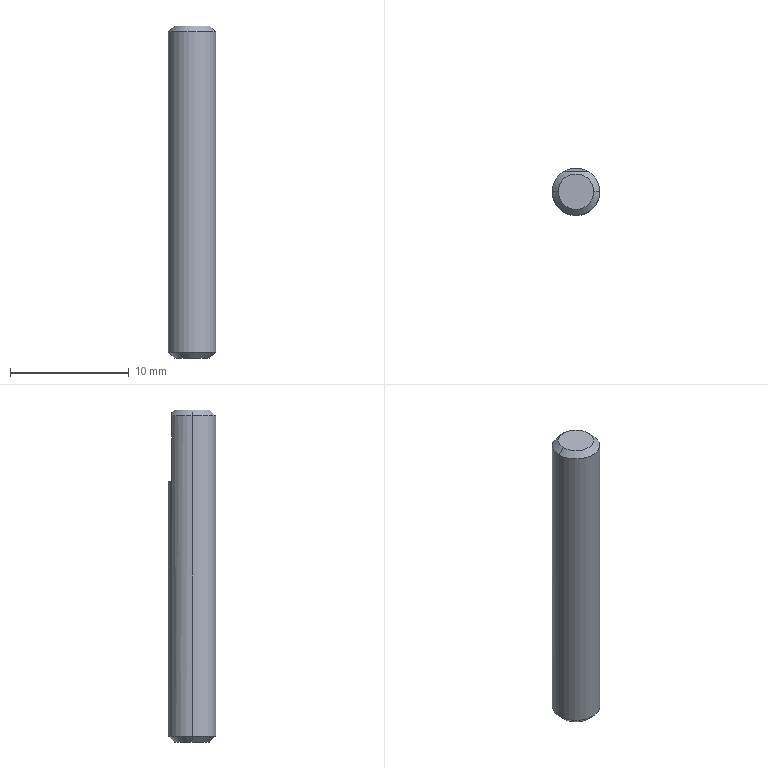Part | SolidWorks | features Chamfer 1, Extrusion 1, ICE 1 | 1 solid | 10 faces | box 4 x 4 x 28 mm | volume 346.573 mm3 | cone 4 | plane 4 | cylinder 2 | commonest cylinder face diameters 4 x2
STEP:
#1=CARTESIAN_POINT('',(1.5,0.,28.));
#2=VERTEX_POINT('',#1);
#3=CARTESIAN_POINT('',(-1.5,0.,28.));
#4=VERTEX_POINT('',#3);
#5=CARTESIAN_POINT('',(0.,0.,28.));
#6=DIRECTION('',(0.,0.,1.));
#7=DIRECTION('',(1.,0.,0.));
#8=AXIS2_PLACEMENT_3D('',#5,#6,#7);
#9=CIRCLE('',#8,1.5);
#10=EDGE_CURVE('',#2,#4,#9,.T.);
#11=ORIENTED_EDGE('',*,*,#10,.F.);
#12=CARTESIAN_POINT('',(2.,0.,27.5));
#13=VERTEX_POINT('',#12);
#14=CARTESIAN_POINT('',(1.5,0.,28.));
#15=DIRECTION('',(0.7071,0.,-0.7071));
#16=VECTOR('',#15,1000.);
#17=LINE('',#14,#16);
#18=EDGE_CURVE('',#2,#13,#17,.T.);
#19=ORIENTED_EDGE('',*,*,#18,.T.);
#20=CARTESIAN_POINT('',(1.054,1.7,27.5));
#21=VERTEX_POINT('',#20);
#22=CARTESIAN_POINT('',(0.,0.,27.5));
#23=DIRECTION('',(0.,0.,-1.));
#24=DIRECTION('',(1.,0.,0.));
#25=AXIS2_PLACEMENT_3D('',#22,#23,#24);
#26=CIRCLE('',#25,2.);
#27=EDGE_CURVE('',#21,#13,#26,.T.);
#28=ORIENTED_EDGE('',*,*,#27,.F.);
#29=CARTESIAN_POINT('',(-1.054,1.7,27.5));
#30=VERTEX_POINT('',#29);
#31=CARTESIAN_POINT('',(-1.054,1.7,27.5));
#32=CARTESIAN_POINT('',(-0.8907,1.7,27.586));
#33=CARTESIAN_POINT('',(-0.7229,1.7,27.66));
#34=CARTESIAN_POINT('',(-0.3692,1.7,27.769));
#35=CARTESIAN_POINT('',(-0.1858,1.7,27.8));
#36=CARTESIAN_POINT('',(0.1827,1.7,27.8));
#37=CARTESIAN_POINT('',(0.368,1.7,27.769));
#38=CARTESIAN_POINT('',(0.7206,1.7,27.661));
#39=CARTESIAN_POINT('',(0.8914,1.7,27.585));
#40=CARTESIAN_POINT('',(1.054,1.7,27.5));
#41=B_SPLINE_CURVE_WITH_KNOTS('',3,(#31,#32,#33,#34,#35,#36,#37,#38,#39,#40),.UNSPECIFIED.,.F.,.F.,(4,2,2,2,4),(0.002731,0.003281,0.003832,0.004382,0.004933),.UNSPECIFIED.);
#42=EDGE_CURVE('',#30,#21,#41,.T.);
#43=ORIENTED_EDGE('',*,*,#42,.F.);
#44=CARTESIAN_POINT('',(-2.,0.,27.5));
#45=VERTEX_POINT('',#44);
#46=CARTESIAN_POINT('',(0.,0.,27.5));
#47=DIRECTION('',(0.,0.,-1.));
#48=DIRECTION('',(1.,0.,0.));
#49=AXIS2_PLACEMENT_3D('',#46,#47,#48);
#50=CIRCLE('',#49,2.);
#51=EDGE_CURVE('',#45,#30,#50,.T.);
#52=ORIENTED_EDGE('',*,*,#51,.F.);
#53=CARTESIAN_POINT('',(-1.5,0.,28.));
#54=DIRECTION('',(-0.7071,0.,-0.7071));
#55=VECTOR('',#54,1000.);
#56=LINE('',#53,#55);
#57=EDGE_CURVE('',#4,#45,#56,.T.);
#58=ORIENTED_EDGE('',*,*,#57,.F.);
#59=EDGE_LOOP('',(#11,#19,#28,#43,#52,#58));
#60=FACE_OUTER_BOUND('',#59,.T.);
#61=CARTESIAN_POINT('',(0.,0.,28.));
#62=DIRECTION('',(0.,0.,-1.));
#63=DIRECTION('',(-1.,0.,0.));
#64=AXIS2_PLACEMENT_3D('',#61,#62,#63);
#65=CONICAL_SURFACE('',#64,1.5,0.7854);
#66=ADVANCED_FACE('',(#60),#65,.T.);
#67=CARTESIAN_POINT('',(-1.5,0.,0.));
#68=VERTEX_POINT('',#67);
#69=CARTESIAN_POINT('',(1.5,0.,0.));
#70=VERTEX_POINT('',#69);
#71=CARTESIAN_POINT('',(0.,0.,0.));
#72=DIRECTION('',(0.,0.,-1.));
#73=DIRECTION('',(1.,0.,0.));
#74=AXIS2_PLACEMENT_3D('',#71,#72,#73);
#75=CIRCLE('',#74,1.5);
#76=EDGE_CURVE('',#68,#70,#75,.T.);
#77=ORIENTED_EDGE('',*,*,#76,.F.);
#78=CARTESIAN_POINT('',(-2.,0.,0.5));
#79=VERTEX_POINT('',#78);
#80=CARTESIAN_POINT('',(-2.,0.,0.5));
#81=DIRECTION('',(-0.7071,0.,0.7071));
#82=VECTOR('',#81,1000.);
#83=LINE('',#80,#82);
#84=EDGE_CURVE('',#68,#79,#83,.T.);
#85=ORIENTED_EDGE('',*,*,#84,.T.);
#86=CARTESIAN_POINT('',(2.,0.,0.5));
#87=VERTEX_POINT('',#86);
#88=CARTESIAN_POINT('',(0.,0.,0.5));
#89=DIRECTION('',(0.,0.,1.));
#90=DIRECTION('',(1.,0.,0.));
#91=AXIS2_PLACEMENT_3D('',#88,#89,#90);
#92=CIRCLE('',#91,2.);
#93=EDGE_CURVE('',#87,#79,#92,.T.);
#94=ORIENTED_EDGE('',*,*,#93,.F.);
#95=CARTESIAN_POINT('',(2.,0.,0.5));
#96=DIRECTION('',(0.7071,0.,0.7071));
#97=VECTOR('',#96,1000.);
#98=LINE('',#95,#97);
#99=EDGE_CURVE('',#70,#87,#98,.T.);
#100=ORIENTED_EDGE('',*,*,#99,.F.);
#101=EDGE_LOOP('',(#77,#85,#94,#100));
#102=FACE_OUTER_BOUND('',#101,.T.);
#103=CARTESIAN_POINT('',(0.,0.,0.5));
#104=DIRECTION('',(0.,0.,1.));
#105=DIRECTION('',(1.,0.,0.));
#106=AXIS2_PLACEMENT_3D('',#103,#104,#105);
#107=CONICAL_SURFACE('',#106,2.,0.7854);
#108=ADVANCED_FACE('',(#102),#107,.T.);
#109=ORIENTED_EDGE('',*,*,#27,.T.);
#110=CARTESIAN_POINT('',(2.,0.,28.));
#111=DIRECTION('',(0.,0.,-1.));
#112=VECTOR('',#111,1000.);
#113=LINE('',#110,#112);
#114=EDGE_CURVE('',#13,#87,#113,.T.);
#115=ORIENTED_EDGE('',*,*,#114,.T.);
#116=ORIENTED_EDGE('',*,*,#93,.T.);
#117=CARTESIAN_POINT('',(-2.,0.,28.));
#118=DIRECTION('',(0.,0.,-1.));
#119=VECTOR('',#118,1000.);
#120=LINE('',#117,#119);
#121=EDGE_CURVE('',#45,#79,#120,.T.);
#122=ORIENTED_EDGE('',*,*,#121,.F.);
#123=ORIENTED_EDGE('',*,*,#51,.T.);
#124=CARTESIAN_POINT('',(-1.054,1.7,22.));
#125=VERTEX_POINT('',#124);
#126=CARTESIAN_POINT('',(-1.054,1.7,28.));
#127=DIRECTION('',(0.,0.,-1.));
#128=VECTOR('',#127,1000.);
#129=LINE('',#126,#128);
#130=EDGE_CURVE('',#30,#125,#129,.T.);
#131=ORIENTED_EDGE('',*,*,#130,.T.);
#132=CARTESIAN_POINT('',(1.054,1.7,22.));
#133=VERTEX_POINT('',#132);
#134=CARTESIAN_POINT('',(0.,0.,22.));
#135=DIRECTION('',(0.,0.,1.));
#136=DIRECTION('',(1.,0.,0.));
#137=AXIS2_PLACEMENT_3D('',#134,#135,#136);
#138=CIRCLE('',#137,2.);
#139=EDGE_CURVE('',#133,#125,#138,.T.);
#140=ORIENTED_EDGE('',*,*,#139,.F.);
#141=CARTESIAN_POINT('',(1.054,1.7,28.));
#142=DIRECTION('',(0.,0.,1.));
#143=VECTOR('',#142,1000.);
#144=LINE('',#141,#143);
#145=EDGE_CURVE('',#133,#21,#144,.T.);
#146=ORIENTED_EDGE('',*,*,#145,.T.);
#147=EDGE_LOOP('',(#109,#115,#116,#122,#123,#131,#140,#146));
#148=FACE_OUTER_BOUND('',#147,.T.);
#149=CARTESIAN_POINT('',(0.,0.,28.));
#150=DIRECTION('',(0.,0.,-1.));
#151=DIRECTION('',(-1.,0.,0.));
#152=AXIS2_PLACEMENT_3D('',#149,#150,#151);
#153=CYLINDRICAL_SURFACE('',#152,2.);
#154=ADVANCED_FACE('',(#148),#153,.T.);
#155=ORIENTED_EDGE('',*,*,#114,.F.);
#156=CARTESIAN_POINT('',(0.,0.,27.5));
#157=DIRECTION('',(0.,0.,-1.));
#158=DIRECTION('',(1.,0.,0.));
#159=AXIS2_PLACEMENT_3D('',#156,#157,#158);
#160=CIRCLE('',#159,2.);
#161=EDGE_CURVE('',#13,#45,#160,.T.);
#162=ORIENTED_EDGE('',*,*,#161,.T.);
#163=ORIENTED_EDGE('',*,*,#121,.T.);
#164=CARTESIAN_POINT('',(0.,0.,0.5));
#165=DIRECTION('',(0.,0.,1.));
#166=DIRECTION('',(1.,0.,0.));
#167=AXIS2_PLACEMENT_3D('',#164,#165,#166);
#168=CIRCLE('',#167,2.);
#169=EDGE_CURVE('',#79,#87,#168,.T.);
#170=ORIENTED_EDGE('',*,*,#169,.T.);
#171=EDGE_LOOP('',(#155,#162,#163,#170));
#172=FACE_OUTER_BOUND('',#171,.T.);
#173=CARTESIAN_POINT('',(0.,0.,28.));
#174=DIRECTION('',(0.,0.,-1.));
#175=DIRECTION('',(-1.,0.,0.));
#176=AXIS2_PLACEMENT_3D('',#173,#174,#175);
#177=CYLINDRICAL_SURFACE('',#176,2.);
#178=ADVANCED_FACE('',(#172),#177,.T.);
#179=CARTESIAN_POINT('',(0.,0.,28.));
#180=DIRECTION('',(0.,0.,1.));
#181=DIRECTION('',(1.,0.,0.));
#182=AXIS2_PLACEMENT_3D('',#179,#180,#181);
#183=CIRCLE('',#182,1.5);
#184=EDGE_CURVE('',#4,#2,#183,.T.);
#185=ORIENTED_EDGE('',*,*,#184,.T.);
#186=ORIENTED_EDGE('',*,*,#10,.T.);
#187=EDGE_LOOP('',(#185,#186));
#188=FACE_OUTER_BOUND('',#187,.T.);
#189=CARTESIAN_POINT('',(0.,0.,28.));
#190=DIRECTION('',(0.,0.,1.));
#191=DIRECTION('',(1.,0.,0.));
#192=AXIS2_PLACEMENT_3D('',#189,#190,#191);
#193=PLANE('',#192);
#194=ADVANCED_FACE('',(#188),#193,.T.);
#195=CARTESIAN_POINT('',(0.,0.,0.));
#196=DIRECTION('',(0.,0.,-1.));
#197=DIRECTION('',(1.,0.,0.));
#198=AXIS2_PLACEMENT_3D('',#195,#196,#197);
#199=CIRCLE('',#198,1.5);
#200=EDGE_CURVE('',#70,#68,#199,.T.);
#201=ORIENTED_EDGE('',*,*,#200,.T.);
#202=ORIENTED_EDGE('',*,*,#76,.T.);
#203=EDGE_LOOP('',(#201,#202));
#204=FACE_OUTER_BOUND('',#203,.T.);
#205=CARTESIAN_POINT('',(0.,0.,0.));
#206=DIRECTION('',(0.,0.,1.));
#207=DIRECTION('',(1.,0.,0.));
#208=AXIS2_PLACEMENT_3D('',#205,#206,#207);
#209=PLANE('',#208);
#210=ADVANCED_FACE('',(#204),#209,.F.);
#211=ORIENTED_EDGE('',*,*,#84,.F.);
#212=ORIENTED_EDGE('',*,*,#200,.F.);
#213=ORIENTED_EDGE('',*,*,#99,.T.);
#214=ORIENTED_EDGE('',*,*,#169,.F.);
#215=EDGE_LOOP('',(#211,#212,#213,#214));
#216=FACE_OUTER_BOUND('',#215,.T.);
#217=CARTESIAN_POINT('',(0.,0.,0.5));
#218=DIRECTION('',(0.,0.,1.));
#219=DIRECTION('',(1.,0.,0.));
#220=AXIS2_PLACEMENT_3D('',#217,#218,#219);
#221=CONICAL_SURFACE('',#220,2.,0.7854);
#222=ADVANCED_FACE('',(#216),#221,.T.);
#223=ORIENTED_EDGE('',*,*,#18,.F.);
#224=ORIENTED_EDGE('',*,*,#184,.F.);
#225=ORIENTED_EDGE('',*,*,#57,.T.);
#226=ORIENTED_EDGE('',*,*,#161,.F.);
#227=EDGE_LOOP('',(#223,#224,#225,#226));
#228=FACE_OUTER_BOUND('',#227,.T.);
#229=CARTESIAN_POINT('',(0.,0.,28.));
#230=DIRECTION('',(0.,0.,-1.));
#231=DIRECTION('',(-1.,0.,0.));
#232=AXIS2_PLACEMENT_3D('',#229,#230,#231);
#233=CONICAL_SURFACE('',#232,1.5,0.7854);
#234=ADVANCED_FACE('',(#228),#233,.T.);
#235=ORIENTED_EDGE('',*,*,#139,.T.);
#236=CARTESIAN_POINT('',(-4.961,1.7,22.));
#237=DIRECTION('',(1.,0.,0.));
#238=VECTOR('',#237,1000.);
#239=LINE('',#236,#238);
#240=EDGE_CURVE('',#125,#133,#239,.T.);
#241=ORIENTED_EDGE('',*,*,#240,.T.);
#242=EDGE_LOOP('',(#235,#241));
#243=FACE_OUTER_BOUND('',#242,.T.);
#244=CARTESIAN_POINT('',(0.,0.,22.));
#245=DIRECTION('',(0.,0.,1.));
#246=DIRECTION('',(1.,0.,0.));
#247=AXIS2_PLACEMENT_3D('',#244,#245,#246);
#248=PLANE('',#247);
#249=ADVANCED_FACE('',(#243),#248,.T.);
#250=ORIENTED_EDGE('',*,*,#42,.T.);
#251=ORIENTED_EDGE('',*,*,#145,.F.);
#252=ORIENTED_EDGE('',*,*,#240,.F.);
#253=ORIENTED_EDGE('',*,*,#130,.F.);
#254=EDGE_LOOP('',(#250,#251,#252,#253));
#255=FACE_OUTER_BOUND('',#254,.T.);
#256=CARTESIAN_POINT('',(-4.961,1.7,22.));
#257=DIRECTION('',(0.,-1.,0.));
#258=DIRECTION('',(0.,0.,-1.));
#259=AXIS2_PLACEMENT_3D('',#256,#257,#258);
#260=PLANE('',#259);
#261=ADVANCED_FACE('',(#255),#260,.F.);
#262=CLOSED_SHELL('',(#66,#108,#154,#178,#194,#210,#222,#234,#249,#261));
#263=MANIFOLD_SOLID_BREP('',#262);
#264=CARTESIAN_POINT('',(0.,0.,0.));
#265=DIRECTION('',(0.,0.,1.));
#266=DIRECTION('',(1.,0.,0.));
#267=AXIS2_PLACEMENT_3D('',#264,#265,#266);
#268=(LENGTH_UNIT()NAMED_UNIT(*)SI_UNIT(.MILLI.,.METRE.));
#269=UNCERTAINTY_MEASURE_WITH_UNIT(LENGTH_MEASURE(0.00001),#268,'','');
#270=(NAMED_UNIT(*)PLANE_ANGLE_UNIT()SI_UNIT($,.RADIAN.));
#271=(NAMED_UNIT(*)SI_UNIT($,.STERADIAN.)SOLID_ANGLE_UNIT());
#272=(GEOMETRIC_REPRESENTATION_CONTEXT(3)GLOBAL_UNCERTAINTY_ASSIGNED_CONTEXT((#269))GLOBAL_UNIT_ASSIGNED_CONTEXT((#268,#270,#271))REPRESENTATION_CONTEXT('',''));
#273=ADVANCED_BREP_SHAPE_REPRESENTATION('',(#263,#267),#272);